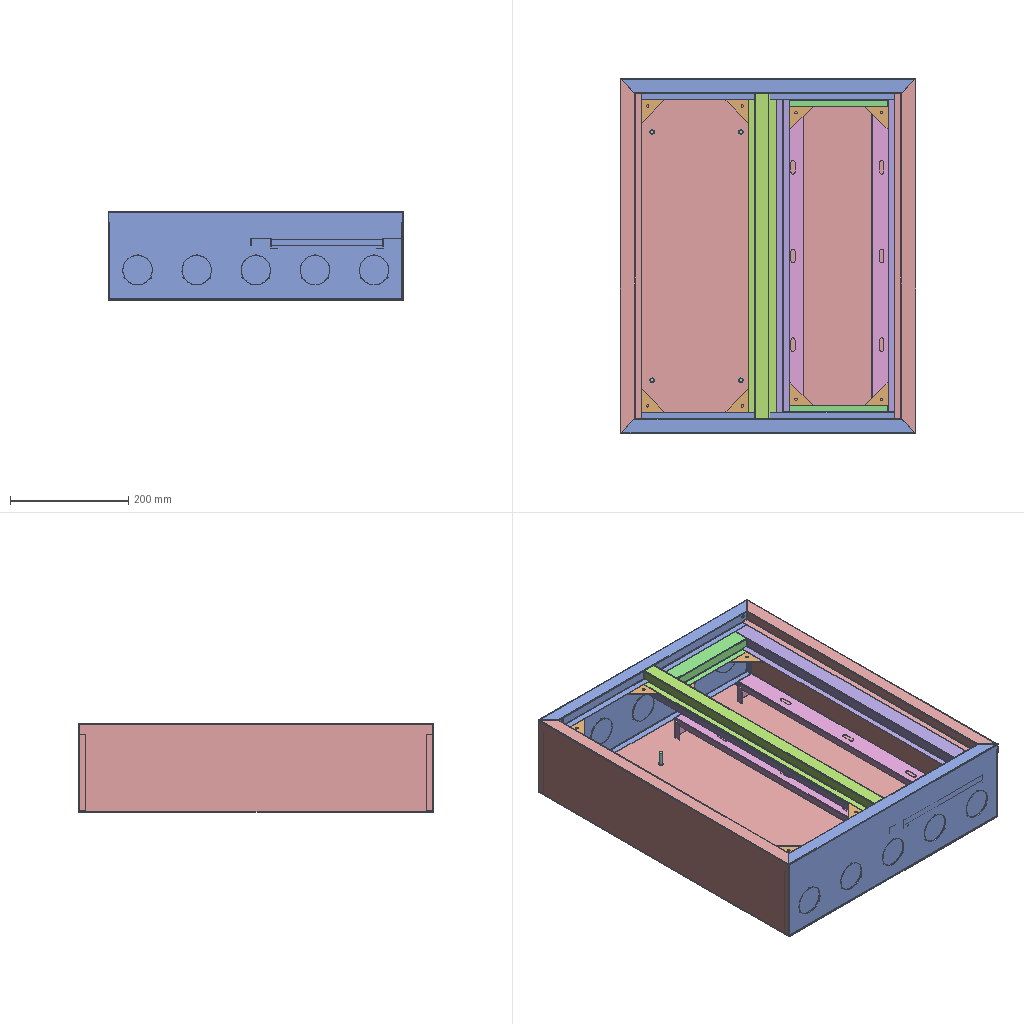Assembly | SolidWorks | 9 different items | 20 placed | box 500 x 600 x 150 mm
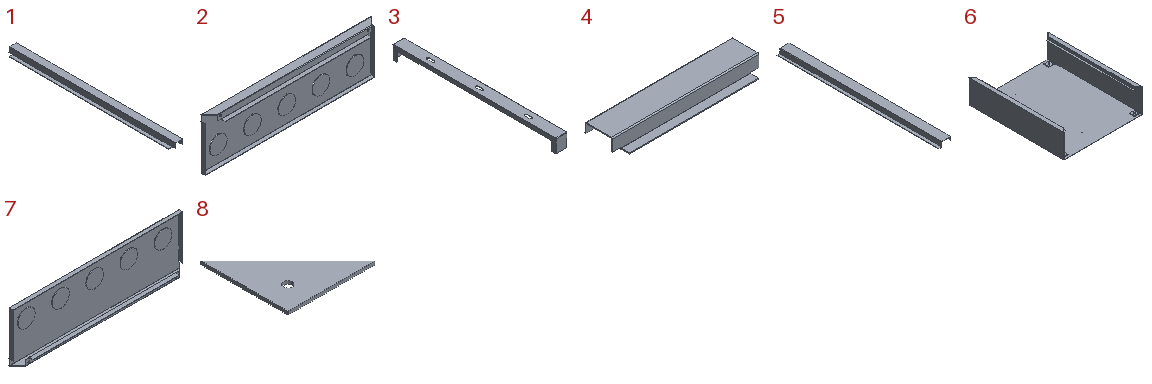Parts list (item | name | quantity | size | volume | features):
1 | - | x1 | 46.6 x 550 x 18 mm | 51368 mm3 | features EdgeFlange 3, FlatPattern 1, ICE 1, SMBaseFlange 1, SheetMetal 1
2 | - | x2 | 497 x 35.8 x 148.8 mm | 125691 mm3 | features EdgeFlange 6, FlatPattern 1, FormToolInstance 1, ICE 1, LPattern 1, SMBaseFlange 1, SheetMetal 1
3 | - | x2 | 35 x 500 x 41 mm | 37614 mm3 | features EdgeFlange 3, FlatPattern 1, SMBaseFlange 1, SheetMetal 1
4 | - | x2 | 188 x 45.8 x 18 mm | 15998 mm3 | features EdgeFlange 3, FlatPattern 1, ICE 1, SMBaseFlange 1, SheetMetal 1
5 | - | x2 | 45.8 x 597 x 18 mm | 51846 mm3 | features EdgeFlange 3, FlatPattern 1, SMBaseFlange 1, SheetMetal 1
6 | - | x1 | 500 x 600 x 150 mm | 642827 mm3 | features EdgeFlange 7, LPattern 3, FormToolInstance 2, FlatPattern 1, ICE 1, SMBaseFlange 1, SheetMetal 1
7 | - | x1 | 497 x 35.8 x 148.8 mm | 125691 mm3 | features MirrorStock 1
8 | - | x8 | 40 x 40 x 1.5 mm | 1179 mm3 | features Cut 1, FlatPattern 1, SMBaseFlange 1, SheetMetal 1
9 | headless studs for stud welding gb | x1 | - | - | -
Mates (type | each side: item.copy, entity, surface, feature):
Coincident | 6.1 face plane Edge-Flange2 | 2.1 face plane Edge-Flange2
DistanceDim | 2.1 face plane Edge-Flange6 | 6.1 face plane Edge-Flange1
Coincident | 6.1 face plane Base-Flange1 | 2.1 face plane Base-Flange1
Coincident | 6.1 face plane Edge-Flange2 | 1.1 face plane Base-Flange1
Coincident | 2.1 face plane Edge-Flange4 | 1.1 face plane Edge-Flange1
DistanceDim | 1.1 face plane Edge-Flange1 | 6.1 face plane Edge-Flange3
Coincident | 6.1 face plane Base-Flange1 | 3.1 face plane Edge-Flange2
DistanceDim | 3.1 face plane Edge-Flange1 | 2.1 face plane Base-Flange1
DistanceDim | 3.1 face plane Edge-Flange2 | 6.1 face plane Edge-Flange1
Coincident | 6.1 face plane Edge-Flange4 | 8.1 face plane Base-Flange1 | 2 times
Coincident | 1.1 face plane Edge-Flange3 | 8.2 face plane Base-Flange1
Coincident | 6.1 face plane Edge-Flange1 | 5.1 face plane Edge-Flange1
DistanceDim | 5.1 face plane Edge-Flange1 | 2.1 face plane Base-Flange1
DistanceDim | 5.1 face plane Base-Flange1 | 6.1 face plane Edge-Flange5
Coincident | 5.1 face plane Base-Flange1 | 4.1 face plane Base-Flange1
Coincident | 5.1 face plane Edge-Flange2 | 4.1 face plane Edge-Flange2
Coincident | 2.1 face plane Base-Flange1 | 4.1 face plane Edge-Flange1
Coincident | 4.1 face plane Base-Flange1 | 5.2 face plane Edge-Flange2
Coincident | 4.1 face plane Base-Flange1 | 5.2 face plane Base-Flange1
DistanceDim | 5.2 face plane Edge-Flange2 | 2.1 face plane Base-Flange1
Coincident | 5.2 face plane Edge-Flange3 | 8.3 face plane Base-Flange1 | 2 times
Coincident | 8.3 face plane Base-Flange1 | 8.4 face plane Base-Flange1
Coincident | 5.1 face plane Edge-Flange3 | 8.4 face plane Base-Flange1
Coincident | 5.1 face plane Base-Flange1 | 4.2 face plane Base-Flange1
Coincident | 5.2 face plane Edge-Flange2 | 4.2 face plane Edge-Flange2
Coincident | 6.1 face plane Base-Flange1 | 2.2 face plane Edge-Flange1
Coincident | 6.1 face plane Edge-Flange1 | 2.2 face plane Edge-Flange3
Coincident | 6.1 face plane Edge-Flange1 | 2.2 face plane Base-Flange1